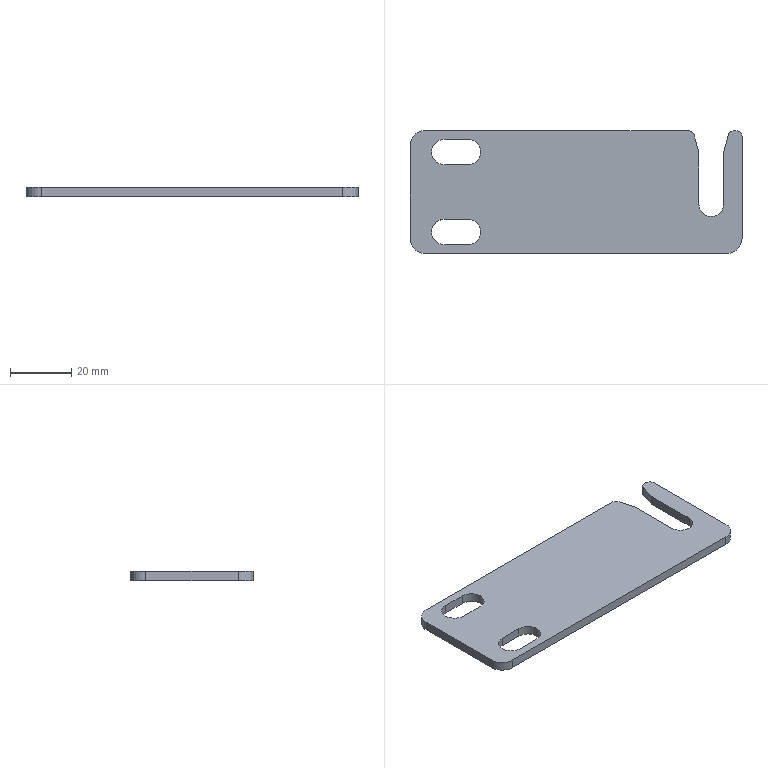Part | SolidWorks | features Fillet 2, Extrusion 1, HoleWzd 1 | 1 solid | 30 faces | box 108 x 40 x 3 mm | volume 11505 mm3 | cylinder 15 | plane 15 | commonest cylinder face diameters 8.3 x6 4 x5 10 x3 8 x1
STEP:
#1=CARTESIAN_POINT('',(-101.,33.,3.));
#2=VERTEX_POINT('',#1);
#3=CARTESIAN_POINT('',(-96.85,37.15,3.));
#4=VERTEX_POINT('',#3);
#5=CARTESIAN_POINT('',(-96.85,33.,3.));
#6=DIRECTION('',(0.,0.,-1.));
#7=DIRECTION('',(-1.,0.,0.));
#8=AXIS2_PLACEMENT_3D('',#5,#6,#7);
#9=CIRCLE('',#8,4.15);
#10=EDGE_CURVE('',#2,#4,#9,.T.);
#11=ORIENTED_EDGE('',*,*,#10,.F.);
#12=CARTESIAN_POINT('',(-101.,33.,0.));
#13=VERTEX_POINT('',#12);
#14=CARTESIAN_POINT('',(-101.,33.,0.));
#15=DIRECTION('',(0.,0.,-1.));
#16=VECTOR('',#15,1000.);
#17=LINE('',#14,#16);
#18=EDGE_CURVE('',#2,#13,#17,.T.);
#19=ORIENTED_EDGE('',*,*,#18,.T.);
#20=CARTESIAN_POINT('',(-96.85,37.15,0.));
#21=VERTEX_POINT('',#20);
#22=CARTESIAN_POINT('',(-96.85,33.,0.));
#23=DIRECTION('',(0.,0.,-1.));
#24=DIRECTION('',(-1.,0.,0.));
#25=AXIS2_PLACEMENT_3D('',#22,#23,#24);
#26=CIRCLE('',#25,4.15);
#27=EDGE_CURVE('',#13,#21,#26,.T.);
#28=ORIENTED_EDGE('',*,*,#27,.T.);
#29=CARTESIAN_POINT('',(-96.85,37.15,0.));
#30=DIRECTION('',(0.,0.,-1.));
#31=VECTOR('',#30,1000.);
#32=LINE('',#29,#31);
#33=EDGE_CURVE('',#4,#21,#32,.T.);
#34=ORIENTED_EDGE('',*,*,#33,.F.);
#35=EDGE_LOOP('',(#11,#19,#28,#34));
#36=FACE_OUTER_BOUND('',#35,.T.);
#37=CARTESIAN_POINT('',(-96.85,33.,0.));
#38=DIRECTION('',(0.,0.,-1.));
#39=DIRECTION('',(-1.,0.,0.));
#40=AXIS2_PLACEMENT_3D('',#37,#38,#39);
#41=CYLINDRICAL_SURFACE('',#40,4.15);
#42=ADVANCED_FACE('',(#36),#41,.F.);
#43=CARTESIAN_POINT('',(-101.,7.,3.));
#44=VERTEX_POINT('',#43);
#45=CARTESIAN_POINT('',(-96.85,11.15,3.));
#46=VERTEX_POINT('',#45);
#47=CARTESIAN_POINT('',(-96.85,7.,3.));
#48=DIRECTION('',(0.,0.,-1.));
#49=DIRECTION('',(-1.,0.,0.));
#50=AXIS2_PLACEMENT_3D('',#47,#48,#49);
#51=CIRCLE('',#50,4.15);
#52=EDGE_CURVE('',#44,#46,#51,.T.);
#53=ORIENTED_EDGE('',*,*,#52,.F.);
#54=CARTESIAN_POINT('',(-101.,7.,0.));
#55=VERTEX_POINT('',#54);
#56=CARTESIAN_POINT('',(-101.,7.,0.));
#57=DIRECTION('',(0.,0.,-1.));
#58=VECTOR('',#57,1000.);
#59=LINE('',#56,#58);
#60=EDGE_CURVE('',#44,#55,#59,.T.);
#61=ORIENTED_EDGE('',*,*,#60,.T.);
#62=CARTESIAN_POINT('',(-96.85,11.15,0.));
#63=VERTEX_POINT('',#62);
#64=CARTESIAN_POINT('',(-96.85,7.,0.));
#65=DIRECTION('',(0.,0.,-1.));
#66=DIRECTION('',(-1.,0.,0.));
#67=AXIS2_PLACEMENT_3D('',#64,#65,#66);
#68=CIRCLE('',#67,4.15);
#69=EDGE_CURVE('',#55,#63,#68,.T.);
#70=ORIENTED_EDGE('',*,*,#69,.T.);
#71=CARTESIAN_POINT('',(-96.85,11.15,0.));
#72=DIRECTION('',(0.,0.,-1.));
#73=VECTOR('',#72,1000.);
#74=LINE('',#71,#73);
#75=EDGE_CURVE('',#46,#63,#74,.T.);
#76=ORIENTED_EDGE('',*,*,#75,.F.);
#77=EDGE_LOOP('',(#53,#61,#70,#76));
#78=FACE_OUTER_BOUND('',#77,.T.);
#79=CARTESIAN_POINT('',(-96.85,7.,0.));
#80=DIRECTION('',(0.,0.,-1.));
#81=DIRECTION('',(-1.,0.,0.));
#82=AXIS2_PLACEMENT_3D('',#79,#80,#81);
#83=CYLINDRICAL_SURFACE('',#82,4.15);
#84=ADVANCED_FACE('',(#78),#83,.F.);
#85=CARTESIAN_POINT('',(-89.15,28.85,3.));
#86=VERTEX_POINT('',#85);
#87=CARTESIAN_POINT('',(-96.85,28.85,3.));
#88=VERTEX_POINT('',#87);
#89=CARTESIAN_POINT('',(-89.15,28.85,3.));
#90=DIRECTION('',(-1.,0.,0.));
#91=VECTOR('',#90,1000.);
#92=LINE('',#89,#91);
#93=EDGE_CURVE('',#86,#88,#92,.T.);
#94=ORIENTED_EDGE('',*,*,#93,.T.);
#95=CARTESIAN_POINT('',(-96.85,33.,3.));
#96=DIRECTION('',(0.,0.,-1.));
#97=DIRECTION('',(-1.,0.,0.));
#98=AXIS2_PLACEMENT_3D('',#95,#96,#97);
#99=CIRCLE('',#98,4.15);
#100=EDGE_CURVE('',#88,#2,#99,.T.);
#101=ORIENTED_EDGE('',*,*,#100,.T.);
#102=ORIENTED_EDGE('',*,*,#10,.T.);
#103=CARTESIAN_POINT('',(-89.15,37.15,3.));
#104=VERTEX_POINT('',#103);
#105=CARTESIAN_POINT('',(-89.15,37.15,3.));
#106=DIRECTION('',(-1.,0.,0.));
#107=VECTOR('',#106,1000.);
#108=LINE('',#105,#107);
#109=EDGE_CURVE('',#104,#4,#108,.T.);
#110=ORIENTED_EDGE('',*,*,#109,.F.);
#111=CARTESIAN_POINT('',(-89.15,33.,3.));
#112=DIRECTION('',(0.,0.,-1.));
#113=DIRECTION('',(-1.,0.,0.));
#114=AXIS2_PLACEMENT_3D('',#111,#112,#113);
#115=CIRCLE('',#114,4.15);
#116=EDGE_CURVE('',#104,#86,#115,.T.);
#117=ORIENTED_EDGE('',*,*,#116,.T.);
#118=EDGE_LOOP('',(#94,#101,#102,#110,#117));
#119=FACE_BOUND('',#118,.T.);
#120=CARTESIAN_POINT('',(-89.15,2.85,3.));
#121=VERTEX_POINT('',#120);
#122=CARTESIAN_POINT('',(-96.85,2.85,3.));
#123=VERTEX_POINT('',#122);
#124=CARTESIAN_POINT('',(-89.15,2.85,3.));
#125=DIRECTION('',(-1.,0.,0.));
#126=VECTOR('',#125,1000.);
#127=LINE('',#124,#126);
#128=EDGE_CURVE('',#121,#123,#127,.T.);
#129=ORIENTED_EDGE('',*,*,#128,.T.);
#130=CARTESIAN_POINT('',(-96.85,7.,3.));
#131=DIRECTION('',(0.,0.,-1.));
#132=DIRECTION('',(-1.,0.,0.));
#133=AXIS2_PLACEMENT_3D('',#130,#131,#132);
#134=CIRCLE('',#133,4.15);
#135=EDGE_CURVE('',#123,#44,#134,.T.);
#136=ORIENTED_EDGE('',*,*,#135,.T.);
#137=ORIENTED_EDGE('',*,*,#52,.T.);
#138=CARTESIAN_POINT('',(-89.15,11.15,3.));
#139=VERTEX_POINT('',#138);
#140=CARTESIAN_POINT('',(-89.15,11.15,3.));
#141=DIRECTION('',(-1.,0.,0.));
#142=VECTOR('',#141,1000.);
#143=LINE('',#140,#142);
#144=EDGE_CURVE('',#139,#46,#143,.T.);
#145=ORIENTED_EDGE('',*,*,#144,.F.);
#146=CARTESIAN_POINT('',(-89.15,7.,3.));
#147=DIRECTION('',(0.,0.,-1.));
#148=DIRECTION('',(-1.,0.,0.));
#149=AXIS2_PLACEMENT_3D('',#146,#147,#148);
#150=CIRCLE('',#149,4.15);
#151=EDGE_CURVE('',#139,#121,#150,.T.);
#152=ORIENTED_EDGE('',*,*,#151,.T.);
#153=EDGE_LOOP('',(#129,#136,#137,#145,#152));
#154=FACE_BOUND('',#153,.T.);
#155=CARTESIAN_POINT('',(-103.,0.,3.));
#156=VERTEX_POINT('',#155);
#157=CARTESIAN_POINT('',(-5.,0.,3.));
#158=VERTEX_POINT('',#157);
#159=CARTESIAN_POINT('',(-108.,0.,3.));
#160=DIRECTION('',(1.,0.,0.));
#161=VECTOR('',#160,1000.);
#162=LINE('',#159,#161);
#163=EDGE_CURVE('',#156,#158,#162,.T.);
#164=ORIENTED_EDGE('',*,*,#163,.T.);
#165=CARTESIAN_POINT('',(0.,5.,3.));
#166=VERTEX_POINT('',#165);
#167=CARTESIAN_POINT('',(-5.,5.,3.));
#168=DIRECTION('',(0.,0.,1.));
#169=DIRECTION('',(-1.,0.,0.));
#170=AXIS2_PLACEMENT_3D('',#167,#168,#169);
#171=CIRCLE('',#170,5.);
#172=EDGE_CURVE('',#158,#166,#171,.T.);
#173=ORIENTED_EDGE('',*,*,#172,.T.);
#174=CARTESIAN_POINT('',(0.,38.,3.));
#175=VERTEX_POINT('',#174);
#176=CARTESIAN_POINT('',(0.,0.,3.));
#177=DIRECTION('',(0.,1.,0.));
#178=VECTOR('',#177,1000.);
#179=LINE('',#176,#178);
#180=EDGE_CURVE('',#166,#175,#179,.T.);
#181=ORIENTED_EDGE('',*,*,#180,.T.);
#182=CARTESIAN_POINT('',(-2.,40.,3.));
#183=VERTEX_POINT('',#182);
#184=CARTESIAN_POINT('',(-2.,38.,3.));
#185=DIRECTION('',(0.,0.,1.));
#186=DIRECTION('',(-1.,0.,0.));
#187=AXIS2_PLACEMENT_3D('',#184,#185,#186);
#188=CIRCLE('',#187,2.);
#189=EDGE_CURVE('',#175,#183,#188,.T.);
#190=ORIENTED_EDGE('',*,*,#189,.T.);
#191=CARTESIAN_POINT('',(-2.491,40.,3.));
#192=VERTEX_POINT('',#191);
#193=CARTESIAN_POINT('',(0.,40.,3.));
#194=DIRECTION('',(-1.,0.,0.));
#195=VECTOR('',#194,1000.);
#196=LINE('',#193,#195);
#197=EDGE_CURVE('',#183,#192,#196,.T.);
#198=ORIENTED_EDGE('',*,*,#197,.T.);
#199=CARTESIAN_POINT('',(-4.414,38.549,3.));
#200=VERTEX_POINT('',#199);
#201=CARTESIAN_POINT('',(-2.491,38.,3.));
#202=DIRECTION('',(0.,0.,1.));
#203=DIRECTION('',(-1.,0.,0.));
#204=AXIS2_PLACEMENT_3D('',#201,#202,#203);
#205=CIRCLE('',#204,2.);
#206=EDGE_CURVE('',#192,#200,#205,.T.);
#207=ORIENTED_EDGE('',*,*,#206,.T.);
#208=CARTESIAN_POINT('',(-5.923,33.269,3.));
#209=VERTEX_POINT('',#208);
#210=CARTESIAN_POINT('',(-4.,40.,3.));
#211=DIRECTION('',(-0.2747,-0.9615,0.));
#212=VECTOR('',#211,1000.);
#213=LINE('',#210,#212);
#214=EDGE_CURVE('',#200,#209,#213,.T.);
#215=ORIENTED_EDGE('',*,*,#214,.T.);
#216=CARTESIAN_POINT('',(-6.,32.72,3.));
#217=VERTEX_POINT('',#216);
#218=CARTESIAN_POINT('',(-4.,32.72,3.));
#219=DIRECTION('',(0.,0.,1.));
#220=DIRECTION('',(-1.,0.,0.));
#221=AXIS2_PLACEMENT_3D('',#218,#219,#220);
#222=CIRCLE('',#221,2.);
#223=EDGE_CURVE('',#209,#217,#222,.T.);
#224=ORIENTED_EDGE('',*,*,#223,.T.);
#225=CARTESIAN_POINT('',(-6.,16.,3.));
#226=VERTEX_POINT('',#225);
#227=CARTESIAN_POINT('',(-6.,33.,3.));
#228=DIRECTION('',(0.,-1.,0.));
#229=VECTOR('',#228,1000.);
#230=LINE('',#227,#229);
#231=EDGE_CURVE('',#217,#226,#230,.T.);
#232=ORIENTED_EDGE('',*,*,#231,.T.);
#233=CARTESIAN_POINT('',(-14.,16.,3.));
#234=VERTEX_POINT('',#233);
#235=CARTESIAN_POINT('',(-10.,16.,3.));
#236=DIRECTION('',(0.,0.,-1.));
#237=DIRECTION('',(-1.,0.,0.));
#238=AXIS2_PLACEMENT_3D('',#235,#236,#237);
#239=CIRCLE('',#238,4.);
#240=EDGE_CURVE('',#226,#234,#239,.T.);
#241=ORIENTED_EDGE('',*,*,#240,.T.);
#242=CARTESIAN_POINT('',(-14.,32.72,3.));
#243=VERTEX_POINT('',#242);
#244=CARTESIAN_POINT('',(-14.,16.,3.));
#245=DIRECTION('',(0.,1.,0.));
#246=VECTOR('',#245,1000.);
#247=LINE('',#244,#246);
#248=EDGE_CURVE('',#234,#243,#247,.T.);
#249=ORIENTED_EDGE('',*,*,#248,.T.);
#250=CARTESIAN_POINT('',(-14.077,33.269,3.));
#251=VERTEX_POINT('',#250);
#252=CARTESIAN_POINT('',(-16.,32.72,3.));
#253=DIRECTION('',(0.,0.,1.));
#254=DIRECTION('',(-1.,0.,0.));
#255=AXIS2_PLACEMENT_3D('',#252,#253,#254);
#256=CIRCLE('',#255,2.);
#257=EDGE_CURVE('',#243,#251,#256,.T.);
#258=ORIENTED_EDGE('',*,*,#257,.T.);
#259=CARTESIAN_POINT('',(-15.586,38.549,3.));
#260=VERTEX_POINT('',#259);
#261=CARTESIAN_POINT('',(-14.,33.,3.));
#262=DIRECTION('',(-0.2747,0.9615,0.));
#263=VECTOR('',#262,1000.);
#264=LINE('',#261,#263);
#265=EDGE_CURVE('',#251,#260,#264,.T.);
#266=ORIENTED_EDGE('',*,*,#265,.T.);
#267=CARTESIAN_POINT('',(-17.509,40.,3.));
#268=VERTEX_POINT('',#267);
#269=CARTESIAN_POINT('',(-17.509,38.,3.));
#270=DIRECTION('',(0.,0.,1.));
#271=DIRECTION('',(-1.,0.,0.));
#272=AXIS2_PLACEMENT_3D('',#269,#270,#271);
#273=CIRCLE('',#272,2.);
#274=EDGE_CURVE('',#260,#268,#273,.T.);
#275=ORIENTED_EDGE('',*,*,#274,.T.);
#276=CARTESIAN_POINT('',(-103.,40.,3.));
#277=VERTEX_POINT('',#276);
#278=CARTESIAN_POINT('',(-16.,40.,3.));
#279=DIRECTION('',(-1.,0.,0.));
#280=VECTOR('',#279,1000.);
#281=LINE('',#278,#280);
#282=EDGE_CURVE('',#268,#277,#281,.T.);
#283=ORIENTED_EDGE('',*,*,#282,.T.);
#284=CARTESIAN_POINT('',(-108.,35.,3.));
#285=VERTEX_POINT('',#284);
#286=CARTESIAN_POINT('',(-103.,35.,3.));
#287=DIRECTION('',(0.,0.,1.));
#288=DIRECTION('',(-1.,0.,0.));
#289=AXIS2_PLACEMENT_3D('',#286,#287,#288);
#290=CIRCLE('',#289,5.);
#291=EDGE_CURVE('',#277,#285,#290,.T.);
#292=ORIENTED_EDGE('',*,*,#291,.T.);
#293=CARTESIAN_POINT('',(-108.,5.,3.));
#294=VERTEX_POINT('',#293);
#295=CARTESIAN_POINT('',(-108.,40.,3.));
#296=DIRECTION('',(0.,-1.,0.));
#297=VECTOR('',#296,1000.);
#298=LINE('',#295,#297);
#299=EDGE_CURVE('',#285,#294,#298,.T.);
#300=ORIENTED_EDGE('',*,*,#299,.T.);
#301=CARTESIAN_POINT('',(-103.,5.,3.));
#302=DIRECTION('',(0.,0.,1.));
#303=DIRECTION('',(-1.,0.,0.));
#304=AXIS2_PLACEMENT_3D('',#301,#302,#303);
#305=CIRCLE('',#304,5.);
#306=EDGE_CURVE('',#294,#156,#305,.T.);
#307=ORIENTED_EDGE('',*,*,#306,.T.);
#308=EDGE_LOOP('',(#164,#173,#181,#190,#198,#207,#215,#224,#232,#241,#249,#258,#266,#275,#283,#292,#300,#307));
#309=FACE_OUTER_BOUND('',#308,.T.);
#310=CARTESIAN_POINT('',(-10.,16.,3.));
#311=DIRECTION('',(0.,0.,-1.));
#312=DIRECTION('',(-1.,0.,0.));
#313=AXIS2_PLACEMENT_3D('',#310,#311,#312);
#314=PLANE('',#313);
#315=ADVANCED_FACE('',(#119,#154,#309),#314,.F.);
#316=CARTESIAN_POINT('',(-89.15,37.15,0.));
#317=VERTEX_POINT('',#316);
#318=CARTESIAN_POINT('',(-89.15,28.85,0.));
#319=VERTEX_POINT('',#318);
#320=CARTESIAN_POINT('',(-89.15,33.,0.));
#321=DIRECTION('',(0.,0.,-1.));
#322=DIRECTION('',(-1.,0.,0.));
#323=AXIS2_PLACEMENT_3D('',#320,#321,#322);
#324=CIRCLE('',#323,4.15);
#325=EDGE_CURVE('',#317,#319,#324,.T.);
#326=ORIENTED_EDGE('',*,*,#325,.F.);
#327=CARTESIAN_POINT('',(-89.15,37.15,0.));
#328=DIRECTION('',(-1.,0.,0.));
#329=VECTOR('',#328,1000.);
#330=LINE('',#327,#329);
#331=EDGE_CURVE('',#317,#21,#330,.T.);
#332=ORIENTED_EDGE('',*,*,#331,.T.);
#333=ORIENTED_EDGE('',*,*,#27,.F.);
#334=CARTESIAN_POINT('',(-96.85,28.85,0.));
#335=VERTEX_POINT('',#334);
#336=CARTESIAN_POINT('',(-96.85,33.,0.));
#337=DIRECTION('',(0.,0.,-1.));
#338=DIRECTION('',(-1.,0.,0.));
#339=AXIS2_PLACEMENT_3D('',#336,#337,#338);
#340=CIRCLE('',#339,4.15);
#341=EDGE_CURVE('',#335,#13,#340,.T.);
#342=ORIENTED_EDGE('',*,*,#341,.F.);
#343=CARTESIAN_POINT('',(-89.15,28.85,0.));
#344=DIRECTION('',(-1.,0.,0.));
#345=VECTOR('',#344,1000.);
#346=LINE('',#343,#345);
#347=EDGE_CURVE('',#319,#335,#346,.T.);
#348=ORIENTED_EDGE('',*,*,#347,.F.);
#349=EDGE_LOOP('',(#326,#332,#333,#342,#348));
#350=FACE_BOUND('',#349,.T.);
#351=CARTESIAN_POINT('',(-89.15,11.15,0.));
#352=VERTEX_POINT('',#351);
#353=CARTESIAN_POINT('',(-89.15,2.85,0.));
#354=VERTEX_POINT('',#353);
#355=CARTESIAN_POINT('',(-89.15,7.,0.));
#356=DIRECTION('',(0.,0.,-1.));
#357=DIRECTION('',(-1.,0.,0.));
#358=AXIS2_PLACEMENT_3D('',#355,#356,#357);
#359=CIRCLE('',#358,4.15);
#360=EDGE_CURVE('',#352,#354,#359,.T.);
#361=ORIENTED_EDGE('',*,*,#360,.F.);
#362=CARTESIAN_POINT('',(-89.15,11.15,0.));
#363=DIRECTION('',(-1.,0.,0.));
#364=VECTOR('',#363,1000.);
#365=LINE('',#362,#364);
#366=EDGE_CURVE('',#352,#63,#365,.T.);
#367=ORIENTED_EDGE('',*,*,#366,.T.);
#368=ORIENTED_EDGE('',*,*,#69,.F.);
#369=CARTESIAN_POINT('',(-96.85,2.85,0.));
#370=VERTEX_POINT('',#369);
#371=CARTESIAN_POINT('',(-96.85,7.,0.));
#372=DIRECTION('',(0.,0.,-1.));
#373=DIRECTION('',(-1.,0.,0.));
#374=AXIS2_PLACEMENT_3D('',#371,#372,#373);
#375=CIRCLE('',#374,4.15);
#376=EDGE_CURVE('',#370,#55,#375,.T.);
#377=ORIENTED_EDGE('',*,*,#376,.F.);
#378=CARTESIAN_POINT('',(-89.15,2.85,0.));
#379=DIRECTION('',(-1.,0.,0.));
#380=VECTOR('',#379,1000.);
#381=LINE('',#378,#380);
#382=EDGE_CURVE('',#354,#370,#381,.T.);
#383=ORIENTED_EDGE('',*,*,#382,.F.);
#384=EDGE_LOOP('',(#361,#367,#368,#377,#383));
#385=FACE_BOUND('',#384,.T.);
#386=CARTESIAN_POINT('',(0.,5.,0.));
#387=VERTEX_POINT('',#386);
#388=CARTESIAN_POINT('',(0.,38.,0.));
#389=VERTEX_POINT('',#388);
#390=CARTESIAN_POINT('',(0.,0.,0.));
#391=DIRECTION('',(0.,1.,0.));
#392=VECTOR('',#391,1000.);
#393=LINE('',#390,#392);
#394=EDGE_CURVE('',#387,#389,#393,.T.);
#395=ORIENTED_EDGE('',*,*,#394,.F.);
#396=CARTESIAN_POINT('',(-5.,0.,0.));
#397=VERTEX_POINT('',#396);
#398=CARTESIAN_POINT('',(-5.,5.,0.));
#399=DIRECTION('',(0.,0.,-1.));
#400=DIRECTION('',(-1.,0.,0.));
#401=AXIS2_PLACEMENT_3D('',#398,#399,#400);
#402=CIRCLE('',#401,5.);
#403=EDGE_CURVE('',#387,#397,#402,.T.);
#404=ORIENTED_EDGE('',*,*,#403,.T.);
#405=CARTESIAN_POINT('',(-103.,0.,0.));
#406=VERTEX_POINT('',#405);
#407=CARTESIAN_POINT('',(-108.,0.,0.));
#408=DIRECTION('',(1.,0.,0.));
#409=VECTOR('',#408,1000.);
#410=LINE('',#407,#409);
#411=EDGE_CURVE('',#406,#397,#410,.T.);
#412=ORIENTED_EDGE('',*,*,#411,.F.);
#413=CARTESIAN_POINT('',(-108.,5.,0.));
#414=VERTEX_POINT('',#413);
#415=CARTESIAN_POINT('',(-103.,5.,0.));
#416=DIRECTION('',(0.,0.,-1.));
#417=DIRECTION('',(-1.,0.,0.));
#418=AXIS2_PLACEMENT_3D('',#415,#416,#417);
#419=CIRCLE('',#418,5.);
#420=EDGE_CURVE('',#406,#414,#419,.T.);
#421=ORIENTED_EDGE('',*,*,#420,.T.);
#422=CARTESIAN_POINT('',(-108.,35.,0.));
#423=VERTEX_POINT('',#422);
#424=CARTESIAN_POINT('',(-108.,40.,0.));
#425=DIRECTION('',(0.,-1.,0.));
#426=VECTOR('',#425,1000.);
#427=LINE('',#424,#426);
#428=EDGE_CURVE('',#423,#414,#427,.T.);
#429=ORIENTED_EDGE('',*,*,#428,.F.);
#430=CARTESIAN_POINT('',(-103.,40.,0.));
#431=VERTEX_POINT('',#430);
#432=CARTESIAN_POINT('',(-103.,35.,0.));
#433=DIRECTION('',(0.,0.,-1.));
#434=DIRECTION('',(-1.,0.,0.));
#435=AXIS2_PLACEMENT_3D('',#432,#433,#434);
#436=CIRCLE('',#435,5.);
#437=EDGE_CURVE('',#423,#431,#436,.T.);
#438=ORIENTED_EDGE('',*,*,#437,.T.);
#439=CARTESIAN_POINT('',(-17.509,40.,0.));
#440=VERTEX_POINT('',#439);
#441=CARTESIAN_POINT('',(-16.,40.,0.));
#442=DIRECTION('',(-1.,0.,0.));
#443=VECTOR('',#442,1000.);
#444=LINE('',#441,#443);
#445=EDGE_CURVE('',#440,#431,#444,.T.);
#446=ORIENTED_EDGE('',*,*,#445,.F.);
#447=CARTESIAN_POINT('',(-15.586,38.549,0.));
#448=VERTEX_POINT('',#447);
#449=CARTESIAN_POINT('',(-17.509,38.,0.));
#450=DIRECTION('',(0.,0.,-1.));
#451=DIRECTION('',(-1.,0.,0.));
#452=AXIS2_PLACEMENT_3D('',#449,#450,#451);
#453=CIRCLE('',#452,2.);
#454=EDGE_CURVE('',#440,#448,#453,.T.);
#455=ORIENTED_EDGE('',*,*,#454,.T.);
#456=CARTESIAN_POINT('',(-14.077,33.269,0.));
#457=VERTEX_POINT('',#456);
#458=CARTESIAN_POINT('',(-14.,33.,0.));
#459=DIRECTION('',(-0.2747,0.9615,0.));
#460=VECTOR('',#459,1000.);
#461=LINE('',#458,#460);
#462=EDGE_CURVE('',#457,#448,#461,.T.);
#463=ORIENTED_EDGE('',*,*,#462,.F.);
#464=CARTESIAN_POINT('',(-14.,32.72,0.));
#465=VERTEX_POINT('',#464);
#466=CARTESIAN_POINT('',(-16.,32.72,0.));
#467=DIRECTION('',(0.,0.,-1.));
#468=DIRECTION('',(-1.,0.,0.));
#469=AXIS2_PLACEMENT_3D('',#466,#467,#468);
#470=CIRCLE('',#469,2.);
#471=EDGE_CURVE('',#457,#465,#470,.T.);
#472=ORIENTED_EDGE('',*,*,#471,.T.);
#473=CARTESIAN_POINT('',(-14.,16.,0.));
#474=VERTEX_POINT('',#473);
#475=CARTESIAN_POINT('',(-14.,16.,0.));
#476=DIRECTION('',(0.,1.,0.));
#477=VECTOR('',#476,1000.);
#478=LINE('',#475,#477);
#479=EDGE_CURVE('',#474,#465,#478,.T.);
#480=ORIENTED_EDGE('',*,*,#479,.F.);
#481=CARTESIAN_POINT('',(-6.,16.,0.));
#482=VERTEX_POINT('',#481);
#483=CARTESIAN_POINT('',(-10.,16.,0.));
#484=DIRECTION('',(0.,0.,-1.));
#485=DIRECTION('',(-1.,0.,0.));
#486=AXIS2_PLACEMENT_3D('',#483,#484,#485);
#487=CIRCLE('',#486,4.);
#488=EDGE_CURVE('',#482,#474,#487,.T.);
#489=ORIENTED_EDGE('',*,*,#488,.F.);
#490=CARTESIAN_POINT('',(-6.,32.72,0.));
#491=VERTEX_POINT('',#490);
#492=CARTESIAN_POINT('',(-6.,33.,0.));
#493=DIRECTION('',(0.,-1.,0.));
#494=VECTOR('',#493,1000.);
#495=LINE('',#492,#494);
#496=EDGE_CURVE('',#491,#482,#495,.T.);
#497=ORIENTED_EDGE('',*,*,#496,.F.);
#498=CARTESIAN_POINT('',(-5.923,33.269,0.));
#499=VERTEX_POINT('',#498);
#500=CARTESIAN_POINT('',(-4.,32.72,0.));
#501=DIRECTION('',(0.,0.,-1.));
#502=DIRECTION('',(-1.,0.,0.));
#503=AXIS2_PLACEMENT_3D('',#500,#501,#502);
#504=CIRCLE('',#503,2.);
#505=EDGE_CURVE('',#491,#499,#504,.T.);
#506=ORIENTED_EDGE('',*,*,#505,.T.);
#507=CARTESIAN_POINT('',(-4.414,38.549,0.));
#508=VERTEX_POINT('',#507);
#509=CARTESIAN_POINT('',(-4.,40.,0.));
#510=DIRECTION('',(-0.2747,-0.9615,0.));
#511=VECTOR('',#510,1000.);
#512=LINE('',#509,#511);
#513=EDGE_CURVE('',#508,#499,#512,.T.);
#514=ORIENTED_EDGE('',*,*,#513,.F.);
#515=CARTESIAN_POINT('',(-2.491,40.,0.));
#516=VERTEX_POINT('',#515);
#517=CARTESIAN_POINT('',(-2.491,38.,0.));
#518=DIRECTION('',(0.,0.,-1.));
#519=DIRECTION('',(-1.,0.,0.));
#520=AXIS2_PLACEMENT_3D('',#517,#518,#519);
#521=CIRCLE('',#520,2.);
#522=EDGE_CURVE('',#508,#516,#521,.T.);
#523=ORIENTED_EDGE('',*,*,#522,.T.);
#524=CARTESIAN_POINT('',(-2.,40.,0.));
#525=VERTEX_POINT('',#524);
#526=CARTESIAN_POINT('',(0.,40.,0.));
#527=DIRECTION('',(-1.,0.,0.));
#528=VECTOR('',#527,1000.);
#529=LINE('',#526,#528);
#530=EDGE_CURVE('',#525,#516,#529,.T.);
#531=ORIENTED_EDGE('',*,*,#530,.F.);
#532=CARTESIAN_POINT('',(-2.,38.,0.));
#533=DIRECTION('',(0.,0.,-1.));
#534=DIRECTION('',(-1.,0.,0.));
#535=AXIS2_PLACEMENT_3D('',#532,#533,#534);
#536=CIRCLE('',#535,2.);
#537=EDGE_CURVE('',#525,#389,#536,.T.);
#538=ORIENTED_EDGE('',*,*,#537,.T.);
#539=EDGE_LOOP('',(#395,#404,#412,#421,#429,#438,#446,#455,#463,#472,#480,#489,#497,#506,#514,#523,#531,#538));
#540=FACE_OUTER_BOUND('',#539,.T.);
#541=CARTESIAN_POINT('',(-10.,16.,0.));
#542=DIRECTION('',(0.,0.,-1.));
#543=DIRECTION('',(-1.,0.,0.));
#544=AXIS2_PLACEMENT_3D('',#541,#542,#543);
#545=PLANE('',#544);
#546=ADVANCED_FACE('',(#350,#385,#540),#545,.T.);
#547=ORIENTED_EDGE('',*,*,#411,.T.);
#548=CARTESIAN_POINT('',(-5.,0.,3.));
#549=DIRECTION('',(0.,0.,1.));
#550=VECTOR('',#549,1000.);
#551=LINE('',#548,#550);
#552=EDGE_CURVE('',#397,#158,#551,.T.);
#553=ORIENTED_EDGE('',*,*,#552,.T.);
#554=ORIENTED_EDGE('',*,*,#163,.F.);
#555=CARTESIAN_POINT('',(-103.,0.,3.));
#556=DIRECTION('',(0.,0.,-1.));
#557=VECTOR('',#556,1000.);
#558=LINE('',#555,#557);
#559=EDGE_CURVE('',#156,#406,#558,.T.);
#560=ORIENTED_EDGE('',*,*,#559,.T.);
#561=EDGE_LOOP('',(#547,#553,#554,#560));
#562=FACE_OUTER_BOUND('',#561,.T.);
#563=CARTESIAN_POINT('',(-108.,0.,3.));
#564=DIRECTION('',(0.,1.,0.));
#565=DIRECTION('',(0.,0.,1.));
#566=AXIS2_PLACEMENT_3D('',#563,#564,#565);
#567=PLANE('',#566);
#568=ADVANCED_FACE('',(#562),#567,.F.);
#569=ORIENTED_EDGE('',*,*,#180,.F.);
#570=CARTESIAN_POINT('',(0.,5.,3.));
#571=DIRECTION('',(0.,0.,-1.));
#572=VECTOR('',#571,1000.);
#573=LINE('',#570,#572);
#574=EDGE_CURVE('',#166,#387,#573,.T.);
#575=ORIENTED_EDGE('',*,*,#574,.T.);
#576=ORIENTED_EDGE('',*,*,#394,.T.);
#577=CARTESIAN_POINT('',(0.,38.,3.));
#578=DIRECTION('',(0.,0.,1.));
#579=VECTOR('',#578,1000.);
#580=LINE('',#577,#579);
#581=EDGE_CURVE('',#389,#175,#580,.T.);
#582=ORIENTED_EDGE('',*,*,#581,.T.);
#583=EDGE_LOOP('',(#569,#575,#576,#582));
#584=FACE_OUTER_BOUND('',#583,.T.);
#585=CARTESIAN_POINT('',(0.,0.,3.));
#586=DIRECTION('',(-1.,0.,0.));
#587=DIRECTION('',(0.,0.,1.));
#588=AXIS2_PLACEMENT_3D('',#585,#586,#587);
#589=PLANE('',#588);
#590=ADVANCED_FACE('',(#584),#589,.F.);
#591=ORIENTED_EDGE('',*,*,#197,.F.);
#592=CARTESIAN_POINT('',(-2.,40.,3.));
#593=DIRECTION('',(0.,0.,-1.));
#594=VECTOR('',#593,1000.);
#595=LINE('',#592,#594);
#596=EDGE_CURVE('',#183,#525,#595,.T.);
#597=ORIENTED_EDGE('',*,*,#596,.T.);
#598=ORIENTED_EDGE('',*,*,#530,.T.);
#599=CARTESIAN_POINT('',(-2.491,40.,3.));
#600=DIRECTION('',(0.,0.,1.));
#601=VECTOR('',#600,1000.);
#602=LINE('',#599,#601);
#603=EDGE_CURVE('',#516,#192,#602,.T.);
#604=ORIENTED_EDGE('',*,*,#603,.T.);
#605=EDGE_LOOP('',(#591,#597,#598,#604));
#606=FACE_OUTER_BOUND('',#605,.T.);
#607=CARTESIAN_POINT('',(0.,40.,3.));
#608=DIRECTION('',(0.,-1.,0.));
#609=DIRECTION('',(0.,0.,-1.));
#610=AXIS2_PLACEMENT_3D('',#607,#608,#609);
#611=PLANE('',#610);
#612=ADVANCED_FACE('',(#606),#611,.F.);
#613=ORIENTED_EDGE('',*,*,#214,.F.);
#614=CARTESIAN_POINT('',(-4.414,38.549,3.));
#615=DIRECTION('',(0.,0.,-1.));
#616=VECTOR('',#615,1000.);
#617=LINE('',#614,#616);
#618=EDGE_CURVE('',#200,#508,#617,.T.);
#619=ORIENTED_EDGE('',*,*,#618,.T.);
#620=ORIENTED_EDGE('',*,*,#513,.T.);
#621=CARTESIAN_POINT('',(-5.923,33.269,3.));
#622=DIRECTION('',(0.,0.,1.));
#623=VECTOR('',#622,1000.);
#624=LINE('',#621,#623);
#625=EDGE_CURVE('',#499,#209,#624,.T.);
#626=ORIENTED_EDGE('',*,*,#625,.T.);
#627=EDGE_LOOP('',(#613,#619,#620,#626));
#628=FACE_OUTER_BOUND('',#627,.T.);
#629=CARTESIAN_POINT('',(-4.,40.,3.));
#630=DIRECTION('',(0.9615,-0.2747,0.));
#631=DIRECTION('',(0.2747,0.9615,0.));
#632=AXIS2_PLACEMENT_3D('',#629,#630,#631);
#633=PLANE('',#632);
#634=ADVANCED_FACE('',(#628),#633,.F.);
#635=ORIENTED_EDGE('',*,*,#231,.F.);
#636=CARTESIAN_POINT('',(-6.,32.72,3.));
#637=DIRECTION('',(0.,0.,-1.));
#638=VECTOR('',#637,1000.);
#639=LINE('',#636,#638);
#640=EDGE_CURVE('',#217,#491,#639,.T.);
#641=ORIENTED_EDGE('',*,*,#640,.T.);
#642=ORIENTED_EDGE('',*,*,#496,.T.);
#643=CARTESIAN_POINT('',(-6.,16.,3.));
#644=DIRECTION('',(0.,0.,-1.));
#645=VECTOR('',#644,1000.);
#646=LINE('',#643,#645);
#647=EDGE_CURVE('',#226,#482,#646,.T.);
#648=ORIENTED_EDGE('',*,*,#647,.F.);
#649=EDGE_LOOP('',(#635,#641,#642,#648));
#650=FACE_OUTER_BOUND('',#649,.T.);
#651=CARTESIAN_POINT('',(-6.,33.,3.));
#652=DIRECTION('',(1.,0.,0.));
#653=DIRECTION('',(0.,1.,0.));
#654=AXIS2_PLACEMENT_3D('',#651,#652,#653);
#655=PLANE('',#654);
#656=ADVANCED_FACE('',(#650),#655,.F.);
#657=ORIENTED_EDGE('',*,*,#488,.T.);
#658=CARTESIAN_POINT('',(-14.,16.,3.));
#659=DIRECTION('',(0.,0.,-1.));
#660=VECTOR('',#659,1000.);
#661=LINE('',#658,#660);
#662=EDGE_CURVE('',#234,#474,#661,.T.);
#663=ORIENTED_EDGE('',*,*,#662,.F.);
#664=ORIENTED_EDGE('',*,*,#240,.F.);
#665=ORIENTED_EDGE('',*,*,#647,.T.);
#666=EDGE_LOOP('',(#657,#663,#664,#665));
#667=FACE_OUTER_BOUND('',#666,.T.);
#668=CARTESIAN_POINT('',(-10.,16.,3.));
#669=DIRECTION('',(0.,0.,-1.));
#670=DIRECTION('',(-1.,0.,0.));
#671=AXIS2_PLACEMENT_3D('',#668,#669,#670);
#672=CYLINDRICAL_SURFACE('',#671,4.);
#673=ADVANCED_FACE('',(#667),#672,.F.);
#674=ORIENTED_EDGE('',*,*,#479,.T.);
#675=CARTESIAN_POINT('',(-14.,32.72,3.));
#676=DIRECTION('',(0.,0.,1.));
#677=VECTOR('',#676,1000.);
#678=LINE('',#675,#677);
#679=EDGE_CURVE('',#465,#243,#678,.T.);
#680=ORIENTED_EDGE('',*,*,#679,.T.);
#681=ORIENTED_EDGE('',*,*,#248,.F.);
#682=ORIENTED_EDGE('',*,*,#662,.T.);
#683=EDGE_LOOP('',(#674,#680,#681,#682));
#684=FACE_OUTER_BOUND('',#683,.T.);
#685=CARTESIAN_POINT('',(-14.,16.,3.));
#686=DIRECTION('',(-1.,0.,0.));
#687=DIRECTION('',(0.,-1.,0.));
#688=AXIS2_PLACEMENT_3D('',#685,#686,#687);
#689=PLANE('',#688);
#690=ADVANCED_FACE('',(#684),#689,.F.);
#691=ORIENTED_EDGE('',*,*,#265,.F.);
#692=CARTESIAN_POINT('',(-14.077,33.269,3.));
#693=DIRECTION('',(0.,0.,-1.));
#694=VECTOR('',#693,1000.);
#695=LINE('',#692,#694);
#696=EDGE_CURVE('',#251,#457,#695,.T.);
#697=ORIENTED_EDGE('',*,*,#696,.T.);
#698=ORIENTED_EDGE('',*,*,#462,.T.);
#699=CARTESIAN_POINT('',(-15.586,38.549,3.));
#700=DIRECTION('',(0.,0.,1.));
#701=VECTOR('',#700,1000.);
#702=LINE('',#699,#701);
#703=EDGE_CURVE('',#448,#260,#702,.T.);
#704=ORIENTED_EDGE('',*,*,#703,.T.);
#705=EDGE_LOOP('',(#691,#697,#698,#704));
#706=FACE_OUTER_BOUND('',#705,.T.);
#707=CARTESIAN_POINT('',(-14.,33.,3.));
#708=DIRECTION('',(-0.9615,-0.2747,0.));
#709=DIRECTION('',(0.2747,-0.9615,0.));
#710=AXIS2_PLACEMENT_3D('',#707,#708,#709);
#711=PLANE('',#710);
#712=ADVANCED_FACE('',(#706),#711,.F.);
#713=ORIENTED_EDGE('',*,*,#445,.T.);
#714=CARTESIAN_POINT('',(-103.,40.,3.));
#715=DIRECTION('',(0.,0.,1.));
#716=VECTOR('',#715,1000.);
#717=LINE('',#714,#716);
#718=EDGE_CURVE('',#431,#277,#717,.T.);
#719=ORIENTED_EDGE('',*,*,#718,.T.);
#720=ORIENTED_EDGE('',*,*,#282,.F.);
#721=CARTESIAN_POINT('',(-17.509,40.,3.));
#722=DIRECTION('',(0.,0.,-1.));
#723=VECTOR('',#722,1000.);
#724=LINE('',#721,#723);
#725=EDGE_CURVE('',#268,#440,#724,.T.);
#726=ORIENTED_EDGE('',*,*,#725,.T.);
#727=EDGE_LOOP('',(#713,#719,#720,#726));
#728=FACE_OUTER_BOUND('',#727,.T.);
#729=CARTESIAN_POINT('',(-16.,40.,3.));
#730=DIRECTION('',(0.,-1.,0.));
#731=DIRECTION('',(0.,0.,-1.));
#732=AXIS2_PLACEMENT_3D('',#729,#730,#731);
#733=PLANE('',#732);
#734=ADVANCED_FACE('',(#728),#733,.F.);
#735=ORIENTED_EDGE('',*,*,#428,.T.);
#736=CARTESIAN_POINT('',(-108.,5.,3.));
#737=DIRECTION('',(0.,0.,1.));
#738=VECTOR('',#737,1000.);
#739=LINE('',#736,#738);
#740=EDGE_CURVE('',#414,#294,#739,.T.);
#741=ORIENTED_EDGE('',*,*,#740,.T.);
#742=ORIENTED_EDGE('',*,*,#299,.F.);
#743=CARTESIAN_POINT('',(-108.,35.,3.));
#744=DIRECTION('',(0.,0.,-1.));
#745=VECTOR('',#744,1000.);
#746=LINE('',#743,#745);
#747=EDGE_CURVE('',#285,#423,#746,.T.);
#748=ORIENTED_EDGE('',*,*,#747,.T.);
#749=EDGE_LOOP('',(#735,#741,#742,#748));
#750=FACE_OUTER_BOUND('',#749,.T.);
#751=CARTESIAN_POINT('',(-108.,40.,3.));
#752=DIRECTION('',(1.,0.,0.));
#753=DIRECTION('',(0.,0.,-1.));
#754=AXIS2_PLACEMENT_3D('',#751,#752,#753);
#755=PLANE('',#754);
#756=ADVANCED_FACE('',(#750),#755,.F.);
#757=ORIENTED_EDGE('',*,*,#60,.F.);
#758=ORIENTED_EDGE('',*,*,#135,.F.);
#759=CARTESIAN_POINT('',(-96.85,2.85,0.));
#760=DIRECTION('',(0.,0.,1.));
#761=VECTOR('',#760,1000.);
#762=LINE('',#759,#761);
#763=EDGE_CURVE('',#370,#123,#762,.T.);
#764=ORIENTED_EDGE('',*,*,#763,.F.);
#765=ORIENTED_EDGE('',*,*,#376,.T.);
#766=EDGE_LOOP('',(#757,#758,#764,#765));
#767=FACE_OUTER_BOUND('',#766,.T.);
#768=CARTESIAN_POINT('',(-96.85,7.,0.));
#769=DIRECTION('',(0.,0.,-1.));
#770=DIRECTION('',(-1.,0.,0.));
#771=AXIS2_PLACEMENT_3D('',#768,#769,#770);
#772=CYLINDRICAL_SURFACE('',#771,4.15);
#773=ADVANCED_FACE('',(#767),#772,.F.);
#774=ORIENTED_EDGE('',*,*,#360,.T.);
#775=CARTESIAN_POINT('',(-89.15,2.85,0.));
#776=DIRECTION('',(0.,0.,-1.));
#777=VECTOR('',#776,1000.);
#778=LINE('',#775,#777);
#779=EDGE_CURVE('',#121,#354,#778,.T.);
#780=ORIENTED_EDGE('',*,*,#779,.F.);
#781=ORIENTED_EDGE('',*,*,#151,.F.);
#782=CARTESIAN_POINT('',(-89.15,11.15,0.));
#783=DIRECTION('',(0.,0.,1.));
#784=VECTOR('',#783,1000.);
#785=LINE('',#782,#784);
#786=EDGE_CURVE('',#352,#139,#785,.T.);
#787=ORIENTED_EDGE('',*,*,#786,.F.);
#788=EDGE_LOOP('',(#774,#780,#781,#787));
#789=FACE_OUTER_BOUND('',#788,.T.);
#790=CARTESIAN_POINT('',(-89.15,7.,0.));
#791=DIRECTION('',(0.,0.,-1.));
#792=DIRECTION('',(-1.,0.,0.));
#793=AXIS2_PLACEMENT_3D('',#790,#791,#792);
#794=CYLINDRICAL_SURFACE('',#793,4.15);
#795=ADVANCED_FACE('',(#789),#794,.F.);
#796=ORIENTED_EDGE('',*,*,#75,.T.);
#797=ORIENTED_EDGE('',*,*,#366,.F.);
#798=ORIENTED_EDGE('',*,*,#786,.T.);
#799=ORIENTED_EDGE('',*,*,#144,.T.);
#800=EDGE_LOOP('',(#796,#797,#798,#799));
#801=FACE_OUTER_BOUND('',#800,.T.);
#802=CARTESIAN_POINT('',(-89.15,11.15,0.));
#803=DIRECTION('',(0.,1.,0.));
#804=DIRECTION('',(0.,0.,1.));
#805=AXIS2_PLACEMENT_3D('',#802,#803,#804);
#806=PLANE('',#805);
#807=ADVANCED_FACE('',(#801),#806,.F.);
#808=ORIENTED_EDGE('',*,*,#763,.T.);
#809=ORIENTED_EDGE('',*,*,#128,.F.);
#810=ORIENTED_EDGE('',*,*,#779,.T.);
#811=ORIENTED_EDGE('',*,*,#382,.T.);
#812=EDGE_LOOP('',(#808,#809,#810,#811));
#813=FACE_OUTER_BOUND('',#812,.T.);
#814=CARTESIAN_POINT('',(-89.15,2.85,0.));
#815=DIRECTION('',(0.,-1.,0.));
#816=DIRECTION('',(0.,0.,-1.));
#817=AXIS2_PLACEMENT_3D('',#814,#815,#816);
#818=PLANE('',#817);
#819=ADVANCED_FACE('',(#813),#818,.F.);
#820=ORIENTED_EDGE('',*,*,#18,.F.);
#821=ORIENTED_EDGE('',*,*,#100,.F.);
#822=CARTESIAN_POINT('',(-96.85,28.85,0.));
#823=DIRECTION('',(0.,0.,1.));
#824=VECTOR('',#823,1000.);
#825=LINE('',#822,#824);
#826=EDGE_CURVE('',#335,#88,#825,.T.);
#827=ORIENTED_EDGE('',*,*,#826,.F.);
#828=ORIENTED_EDGE('',*,*,#341,.T.);
#829=EDGE_LOOP('',(#820,#821,#827,#828));
#830=FACE_OUTER_BOUND('',#829,.T.);
#831=CARTESIAN_POINT('',(-96.85,33.,0.));
#832=DIRECTION('',(0.,0.,-1.));
#833=DIRECTION('',(-1.,0.,0.));
#834=AXIS2_PLACEMENT_3D('',#831,#832,#833);
#835=CYLINDRICAL_SURFACE('',#834,4.15);
#836=ADVANCED_FACE('',(#830),#835,.F.);
#837=ORIENTED_EDGE('',*,*,#325,.T.);
#838=CARTESIAN_POINT('',(-89.15,28.85,0.));
#839=DIRECTION('',(0.,0.,-1.));
#840=VECTOR('',#839,1000.);
#841=LINE('',#838,#840);
#842=EDGE_CURVE('',#86,#319,#841,.T.);
#843=ORIENTED_EDGE('',*,*,#842,.F.);
#844=ORIENTED_EDGE('',*,*,#116,.F.);
#845=CARTESIAN_POINT('',(-89.15,37.15,0.));
#846=DIRECTION('',(0.,0.,1.));
#847=VECTOR('',#846,1000.);
#848=LINE('',#845,#847);
#849=EDGE_CURVE('',#317,#104,#848,.T.);
#850=ORIENTED_EDGE('',*,*,#849,.F.);
#851=EDGE_LOOP('',(#837,#843,#844,#850));
#852=FACE_OUTER_BOUND('',#851,.T.);
#853=CARTESIAN_POINT('',(-89.15,33.,0.));
#854=DIRECTION('',(0.,0.,-1.));
#855=DIRECTION('',(-1.,0.,0.));
#856=AXIS2_PLACEMENT_3D('',#853,#854,#855);
#857=CYLINDRICAL_SURFACE('',#856,4.15);
#858=ADVANCED_FACE('',(#852),#857,.F.);
#859=ORIENTED_EDGE('',*,*,#33,.T.);
#860=ORIENTED_EDGE('',*,*,#331,.F.);
#861=ORIENTED_EDGE('',*,*,#849,.T.);
#862=ORIENTED_EDGE('',*,*,#109,.T.);
#863=EDGE_LOOP('',(#859,#860,#861,#862));
#864=FACE_OUTER_BOUND('',#863,.T.);
#865=CARTESIAN_POINT('',(-89.15,37.15,0.));
#866=DIRECTION('',(0.,1.,0.));
#867=DIRECTION('',(0.,0.,1.));
#868=AXIS2_PLACEMENT_3D('',#865,#866,#867);
#869=PLANE('',#868);
#870=ADVANCED_FACE('',(#864),#869,.F.);
#871=ORIENTED_EDGE('',*,*,#826,.T.);
#872=ORIENTED_EDGE('',*,*,#93,.F.);
#873=ORIENTED_EDGE('',*,*,#842,.T.);
#874=ORIENTED_EDGE('',*,*,#347,.T.);
#875=EDGE_LOOP('',(#871,#872,#873,#874));
#876=FACE_OUTER_BOUND('',#875,.T.);
#877=CARTESIAN_POINT('',(-89.15,28.85,0.));
#878=DIRECTION('',(0.,-1.,0.));
#879=DIRECTION('',(0.,0.,-1.));
#880=AXIS2_PLACEMENT_3D('',#877,#878,#879);
#881=PLANE('',#880);
#882=ADVANCED_FACE('',(#876),#881,.F.);
#883=ORIENTED_EDGE('',*,*,#189,.F.);
#884=ORIENTED_EDGE('',*,*,#581,.F.);
#885=ORIENTED_EDGE('',*,*,#537,.F.);
#886=ORIENTED_EDGE('',*,*,#596,.F.);
#887=EDGE_LOOP('',(#883,#884,#885,#886));
#888=FACE_OUTER_BOUND('',#887,.T.);
#889=CARTESIAN_POINT('',(-2.,38.,3.));
#890=DIRECTION('',(0.,0.,-1.));
#891=DIRECTION('',(-1.,0.,0.));
#892=AXIS2_PLACEMENT_3D('',#889,#890,#891);
#893=CYLINDRICAL_SURFACE('',#892,2.);
#894=ADVANCED_FACE('',(#888),#893,.T.);
#895=ORIENTED_EDGE('',*,*,#206,.F.);
#896=ORIENTED_EDGE('',*,*,#603,.F.);
#897=ORIENTED_EDGE('',*,*,#522,.F.);
#898=ORIENTED_EDGE('',*,*,#618,.F.);
#899=EDGE_LOOP('',(#895,#896,#897,#898));
#900=FACE_OUTER_BOUND('',#899,.T.);
#901=CARTESIAN_POINT('',(-2.491,38.,3.));
#902=DIRECTION('',(0.,0.,-1.));
#903=DIRECTION('',(-1.,0.,0.));
#904=AXIS2_PLACEMENT_3D('',#901,#902,#903);
#905=CYLINDRICAL_SURFACE('',#904,2.);
#906=ADVANCED_FACE('',(#900),#905,.T.);
#907=ORIENTED_EDGE('',*,*,#223,.F.);
#908=ORIENTED_EDGE('',*,*,#625,.F.);
#909=ORIENTED_EDGE('',*,*,#505,.F.);
#910=ORIENTED_EDGE('',*,*,#640,.F.);
#911=EDGE_LOOP('',(#907,#908,#909,#910));
#912=FACE_OUTER_BOUND('',#911,.T.);
#913=CARTESIAN_POINT('',(-4.,32.72,3.));
#914=DIRECTION('',(0.,0.,-1.));
#915=DIRECTION('',(-1.,0.,0.));
#916=AXIS2_PLACEMENT_3D('',#913,#914,#915);
#917=CYLINDRICAL_SURFACE('',#916,2.);
#918=ADVANCED_FACE('',(#912),#917,.T.);
#919=ORIENTED_EDGE('',*,*,#257,.F.);
#920=ORIENTED_EDGE('',*,*,#679,.F.);
#921=ORIENTED_EDGE('',*,*,#471,.F.);
#922=ORIENTED_EDGE('',*,*,#696,.F.);
#923=EDGE_LOOP('',(#919,#920,#921,#922));
#924=FACE_OUTER_BOUND('',#923,.T.);
#925=CARTESIAN_POINT('',(-16.,32.72,3.));
#926=DIRECTION('',(0.,0.,-1.));
#927=DIRECTION('',(-1.,0.,0.));
#928=AXIS2_PLACEMENT_3D('',#925,#926,#927);
#929=CYLINDRICAL_SURFACE('',#928,2.);
#930=ADVANCED_FACE('',(#924),#929,.T.);
#931=ORIENTED_EDGE('',*,*,#274,.F.);
#932=ORIENTED_EDGE('',*,*,#703,.F.);
#933=ORIENTED_EDGE('',*,*,#454,.F.);
#934=ORIENTED_EDGE('',*,*,#725,.F.);
#935=EDGE_LOOP('',(#931,#932,#933,#934));
#936=FACE_OUTER_BOUND('',#935,.T.);
#937=CARTESIAN_POINT('',(-17.509,38.,3.));
#938=DIRECTION('',(0.,0.,-1.));
#939=DIRECTION('',(-1.,0.,0.));
#940=AXIS2_PLACEMENT_3D('',#937,#938,#939);
#941=CYLINDRICAL_SURFACE('',#940,2.);
#942=ADVANCED_FACE('',(#936),#941,.T.);
#943=ORIENTED_EDGE('',*,*,#172,.F.);
#944=ORIENTED_EDGE('',*,*,#552,.F.);
#945=ORIENTED_EDGE('',*,*,#403,.F.);
#946=ORIENTED_EDGE('',*,*,#574,.F.);
#947=EDGE_LOOP('',(#943,#944,#945,#946));
#948=FACE_OUTER_BOUND('',#947,.T.);
#949=CARTESIAN_POINT('',(-5.,5.,3.));
#950=DIRECTION('',(0.,0.,-1.));
#951=DIRECTION('',(-1.,0.,0.));
#952=AXIS2_PLACEMENT_3D('',#949,#950,#951);
#953=CYLINDRICAL_SURFACE('',#952,5.);
#954=ADVANCED_FACE('',(#948),#953,.T.);
#955=ORIENTED_EDGE('',*,*,#306,.F.);
#956=ORIENTED_EDGE('',*,*,#740,.F.);
#957=ORIENTED_EDGE('',*,*,#420,.F.);
#958=ORIENTED_EDGE('',*,*,#559,.F.);
#959=EDGE_LOOP('',(#955,#956,#957,#958));
#960=FACE_OUTER_BOUND('',#959,.T.);
#961=CARTESIAN_POINT('',(-103.,5.,3.));
#962=DIRECTION('',(0.,0.,-1.));
#963=DIRECTION('',(-1.,0.,0.));
#964=AXIS2_PLACEMENT_3D('',#961,#962,#963);
#965=CYLINDRICAL_SURFACE('',#964,5.);
#966=ADVANCED_FACE('',(#960),#965,.T.);
#967=ORIENTED_EDGE('',*,*,#291,.F.);
#968=ORIENTED_EDGE('',*,*,#718,.F.);
#969=ORIENTED_EDGE('',*,*,#437,.F.);
#970=ORIENTED_EDGE('',*,*,#747,.F.);
#971=EDGE_LOOP('',(#967,#968,#969,#970));
#972=FACE_OUTER_BOUND('',#971,.T.);
#973=CARTESIAN_POINT('',(-103.,35.,3.));
#974=DIRECTION('',(0.,0.,-1.));
#975=DIRECTION('',(-1.,0.,0.));
#976=AXIS2_PLACEMENT_3D('',#973,#974,#975);
#977=CYLINDRICAL_SURFACE('',#976,5.);
#978=ADVANCED_FACE('',(#972),#977,.T.);
#979=CLOSED_SHELL('',(#42,#84,#315,#546,#568,#590,#612,#634,#656,#673,#690,#712,#734,#756,#773,#795,#807,#819,#836,#858,#870,#882,#894,#906,#918,#930,#942,#954,#966,#978));
#980=MANIFOLD_SOLID_BREP('',#979);
#981=CARTESIAN_POINT('',(0.,0.,0.));
#982=DIRECTION('',(0.,0.,1.));
#983=DIRECTION('',(1.,0.,0.));
#984=AXIS2_PLACEMENT_3D('',#981,#982,#983);
#985=(LENGTH_UNIT()NAMED_UNIT(*)SI_UNIT(.MILLI.,.METRE.));
#986=UNCERTAINTY_MEASURE_WITH_UNIT(LENGTH_MEASURE(0.00001),#985,'','');
#987=(NAMED_UNIT(*)PLANE_ANGLE_UNIT()SI_UNIT($,.RADIAN.));
#988=(NAMED_UNIT(*)SI_UNIT($,.STERADIAN.)SOLID_ANGLE_UNIT());
#989=(GEOMETRIC_REPRESENTATION_CONTEXT(3)GLOBAL_UNCERTAINTY_ASSIGNED_CONTEXT((#986))GLOBAL_UNIT_ASSIGNED_CONTEXT((#985,#987,#988))REPRESENTATION_CONTEXT('',''));
#990=ADVANCED_BREP_SHAPE_REPRESENTATION('',(#980,#984),#989);